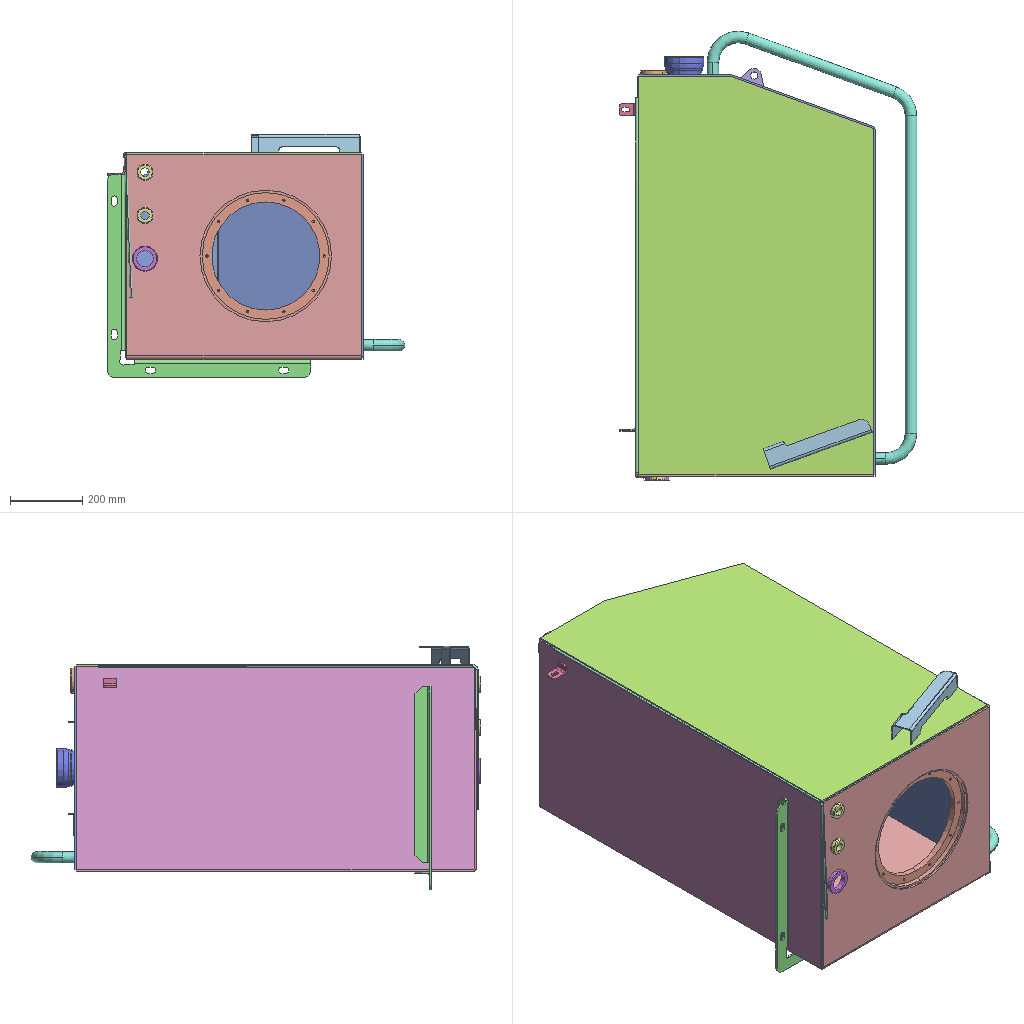Assembly | SolidWorks | 24 different items | 26 placed | box 826 x 1248 x 675 mm
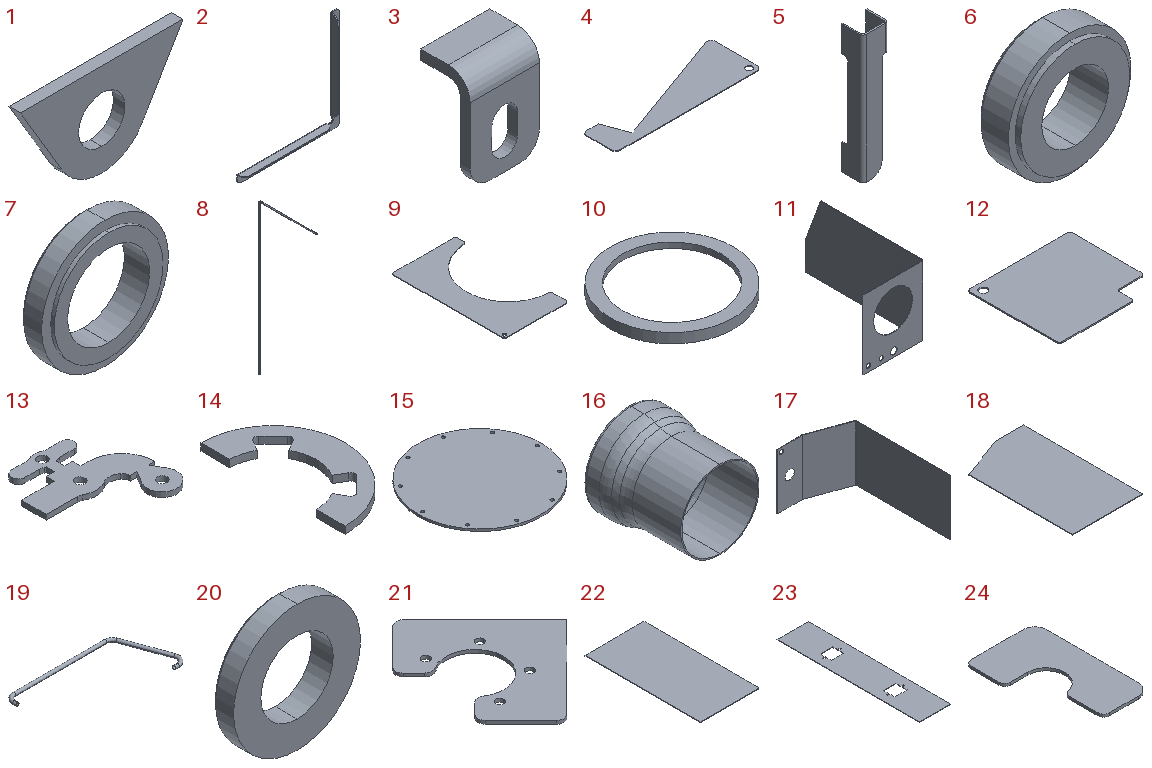Parts list (item | quantity | size | volume | features):
1 | x2 | 70 x 5 x 40 mm | 7506 mm3 | features FlatPattern 1, SMBaseFlange 1, SheetMetal 1
2 | x1 | 565 x 45.004 x 565 mm | 429938 mm3 | features FlatPattern 1, SM3dBend 1, SMBaseFlange 1, SheetMetal 1, UnFold 1
3 | x1 | 35 x 25 x 50 mm | 10083 mm3 | features Fillet 1, FlatPattern 1, ICE 1, SMBaseFlange 1, SheetMetal 1, UnFold 1
4 | x1 | 350 x 121.27 x 1.6 mm | 39939 mm3 | features FlatPattern 1, SMBaseFlange 1, SheetMetal 1
5 | x1 | 60 x 50 x 300 mm | 82869 mm3 | features ICE 2, Fillet 1, FlatPattern 1, SMBaseFlange 1, SheetMetal 1, UnFold 1
6 | x2 | 45 x 14 x 45 mm | 14724 mm3 | features HoleWzd 1, Revolution 1
7 | x1 | 70 x 14 x 70 mm | 28891 mm3 | features HoleWzd 1, Revolution 1
8 | x1 | 8 x 404 x 1054 mm | 31793 mm3 | features Sweep 1
9 | x1 | 283 x 500 x 2.3 mm | 197741 mm3 | features FlatPattern 1, SMBaseFlange 1, SheetMetal 1
10 | x1 | 375 x 375 x 30 mm | 842431 mm3 | features HoleWzd 1, Revolution 1
11 | x1 | 570.5 x 1110 x 651 mm | 4749925 mm3 | features ICE 2, Fillet 1, FlatPattern 1, SMBaseFlange 1, SheetMetal 1, UnFold 1
12 | x1 | 130 x 116.815 x 1.6 mm | 22938 mm3 | features FlatPattern 1, SMBaseFlange 1, SheetMetal 1
13 | x1 | 62.5 x 61.5 x 3 mm | 4665 mm3 | features FlatPattern 1, ICE 1, SMBaseFlange 1, SheetMetal 1
14 | x1 | 80 x 160 x 8 mm | 42936 mm3 | features FlatPattern 1, SMBaseFlange 1, SheetMetal 1
15 | x1 | 350 x 350 x 6 mm | 573863 mm3 | features BaseBody 1
16 | x1 | 110 x 112 x 110 mm | 57636 mm3 | features CirPattern 1, ICE 1, Revolution 1
17 | x1 | 655 x 1110 x 565 mm | 4586470 mm3 | features Fillet 1, FlatPattern 1, ICE 1, SMBaseFlange 1, SheetMetal 1, UnFold 1
18 | x1 | 651 x 1106 x 5 mm | 3454699 mm3 | features Extrusion 1, Fillet 1
19 | x1 | 1202 x 582 x 32 mm | 468025 mm3 | features Sweep 1
20 | x1 | 70 x 12 x 70 mm | 29948 mm3 | features HoleWzd 1, ICE 1, Revolution 1
21 | x1 | 89.853 x 116.066 x 2.3 mm | 10484 mm3 | features FlatPattern 1, SMBaseFlange 1, SheetMetal 1
22 | x1 | 565 x 1106 x 5 mm | 3122985 mm3 | features Fillet 1, FlatPattern 1, SMBaseFlange 1, SheetMetal 1
23 | x1 | 125 x 575 x 1.6 mm | 107480 mm3 | features FlatPattern 1, SMBaseFlange 1, SheetMetal 1
24 | x1 | 60 x 100 x 2.3 mm | 9695 mm3 | features FlatPattern 1, SMBaseFlange 1, SheetMetal 1
Mates (type | each side: item.copy, entity, surface, feature):
Coincident | 11.1 face plane Base-Flange1 | 17.1 face plane Base-Flange1 | 2 times
DistanceDim | 11.1 face plane Base-Flange1 | 17.1 face plane Base-Flange1
Coincident | 17.1 face plane Base-Flange1 | 18.1 face plane Boss-Extrude1
Coincident | 11.1 face plane Base-Flange1 | 18.1 face plane Boss-Extrude1 | 2 times
Coincident | 11.1 face plane Base-Flange1 | 22.1 face plane Base-Flange1 | 2 times
Coincident | 17.1 face plane Base-Flange1 | 22.1 face plane Base-Flange1
Coincident | 17.1 face plane Base-Flange1 | 19.1 face plane Sweep1 | 2 times
DistanceDim | 19.1 face cylinder Sweep1 | 11.1 face plane Base-Flange1
Coincident | 17.1 face plane Base-Flange1 | 20.1 face plane Revolve1
Concentric | 17.1 face cylinder Cut-Extrude1 | 20.1 face cylinder Revolve1
PlanarAngleDim | 20.1 plane | assembly plane
Coincident | 17.1 face plane Base-Flange1 | 1.1 face plane Base-Flange1
DistanceDim | 1.1 plane | 17.1 plane
DistanceDim | 1.1 face cylinder Base-Flange1 | 22.1 face plane Base-Flange1
Coincident | 22.1 face plane Base-Flange1 | 2.1 face plane Base-Flange1
Coincident | 11.1 face plane Base-Flange1 | 2.1 face plane Base-Flange1
DistanceDim | 2.1 face plane Base-Flange1 | 11.1 face plane Base-Flange1
Coincident | 22.1 face plane Base-Flange1 | 3.1 face plane Base-Flange1
DistanceDim | 3.1 face plane Base-Flange1 | 18.1 face plane Boss-Extrude1
DistanceDim | 3.1 face plane Base-Flange1 | 11.1 face plane Base-Flange1
Coincident | 18.1 face plane Boss-Extrude1 | 5.1 face plane Base-Flange1
PlanarAngleDim | 5.1 face plane Base-Flange1 | 11.1 face plane Base-Flange1
DistanceDim | 5.1 edge | 22.1 face plane Base-Flange1
DistanceDim | 5.1 edge | 11.1 face plane Base-Flange1
Coincident | 11.1 face plane Base-Flange1 | 6.1 face plane Revolve1
Concentric | 11.1 face cylinder Cut-Extrude2 | 6.1 face cylinder G3/4 Tapped Hole1
Parallel | 6.1 plane | assembly plane
Coincident | 11.1 face plane Base-Flange1 | 6.2 face plane Revolve1
Concentric | 11.1 face cylinder Cut-Extrude2 | 6.2 face cylinder G3/4 Tapped Hole1
Parallel | 6.2 plane | assembly plane
Coincident | 11.1 face plane Base-Flange1 | 7.1 face plane Revolve1
Concentric | 11.1 face cylinder Cut-Extrude2 | 7.1 face cylinder G1-1/2 Tapped Hole1
Parallel | 7.1 plane | assembly plane
DistanceDim | 22.1 face plane Base-Flange1 | 8.1 face cylinder Sweep1
DistanceDim | 11.1 face plane Base-Flange1 | 8.1 face cylinder Sweep1
Concentric | 17.1 face cylinder Cut-Extrude1 | 16.1 face cylinder Revolve1
DistanceDim | 16.1 face plane Revolve1 | 17.1 face plane Base-Flange1
Coincident | 17.1 face plane Base-Flange1 | 13.1 face plane Base-Flange1
DistanceDim | 13.1 face plane Base-Flange1 | 11.1 face plane Base-Flange1
DistanceDim | 22.1 face plane Base-Flange1 | 13.1 face plane Base-Flange1
InPlace | 18.1 face plane Boss-Extrude1 | 4.1 plane
InPlace | 17.1 face plane Base-Flange1 | 23.1 plane
InPlace | 17.1 face plane Base-Flange1 | 12.1 plane
Tangent | 18.1 face plane Boss-Extrude1 | 8.1 face cylinder Sweep1
InPlace | 11.1 face plane Base-Flange1 | 9.1 plane
InPlace | 17.1 face plane Base-Flange1 | 14.1 plane
InPlace | 20.1 face plane Revolve1 | 21.1 plane
Coincident | 11.1 face plane Base-Flange1 | 10.1 face plane Revolve1
Concentric | 11.1 face cylinder Cut-Extrude2 | 10.1 face cylinder Revolve1
Coincident | 10.1 face plane Revolve1 | 15.1 face plane Import1
Concentric | 10.1 face cylinder M8 Tapped Hole1 | 15.1 face cylinder Import1 | 2 times
Parallel | 10.1 plane | assembly plane
InPlace | 17.1 face plane Base-Flange1 | 24.1 plane